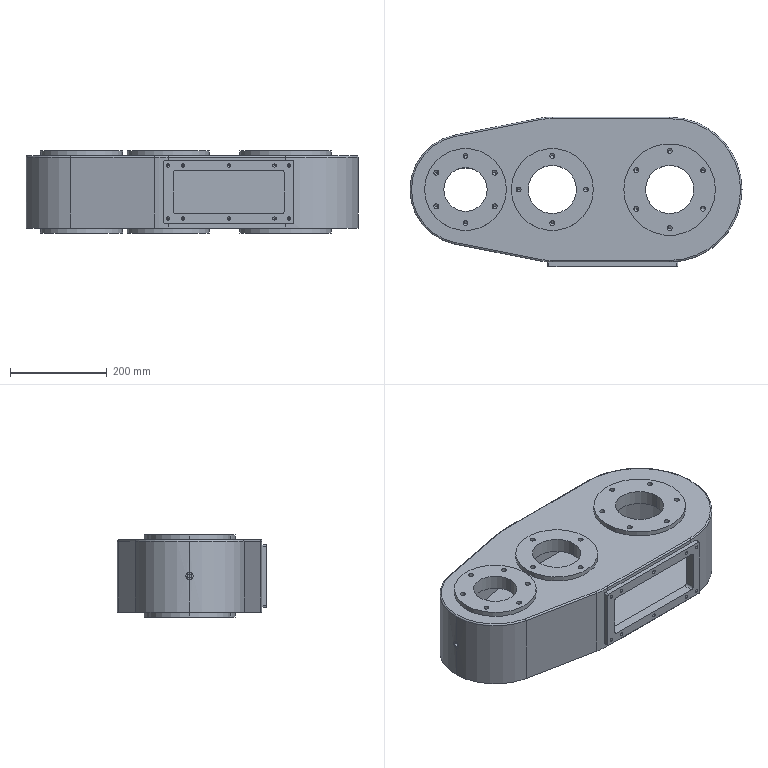Part | SolidWorks | features 3DProfileFeature 6, HoleWzd 6, ICE 6, CirPattern 4, Fillet 3, MirrorPattern 3, Cut 1, Extrusion 1 | 1 solid | 252 faces | box 688 x 310 x 170 mm | volume 8954968 mm3 | cylinder 136 | cone 80 | plane 31 | torus 5 | commonest cylinder face diameters 10.2 x60 6.8 x26 6 x8 100 x8 170 x8 10 x4